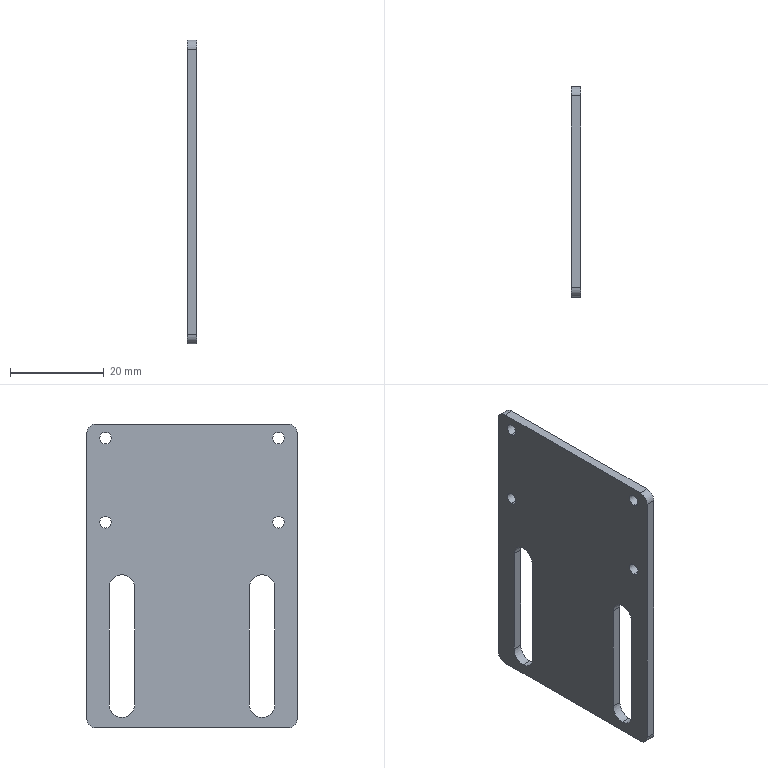Part | SolidWorks | features Fillet 1, FlatPattern 1, HoleWzd 1, ICE 1, SMBaseFlange 1, SheetMetal 1 | 1 solid | 28 faces | box 2 x 45 x 65 mm | volume 5159 mm3 | cylinder 18 | plane 10 | commonest cylinder face diameters 2.5 x8 5.5 x6 4 x4
STEP:
#1=CARTESIAN_POINT('',(-2.,18.5,30.75));
#2=VERTEX_POINT('',#1);
#3=CARTESIAN_POINT('',(-2.,18.5,28.25));
#4=VERTEX_POINT('',#3);
#5=CARTESIAN_POINT('',(-2.,18.5,29.5));
#6=DIRECTION('',(1.,0.,0.));
#7=DIRECTION('',(0.,0.,-1.));
#8=AXIS2_PLACEMENT_3D('',#5,#6,#7);
#9=CIRCLE('',#8,1.25);
#10=EDGE_CURVE('',#2,#4,#9,.T.);
#11=ORIENTED_EDGE('',*,*,#10,.F.);
#12=CARTESIAN_POINT('',(0.,18.5,30.75));
#13=VERTEX_POINT('',#12);
#14=CARTESIAN_POINT('',(0.,18.5,30.75));
#15=DIRECTION('',(1.,0.,0.));
#16=VECTOR('',#15,1000.);
#17=LINE('',#14,#16);
#18=EDGE_CURVE('',#2,#13,#17,.T.);
#19=ORIENTED_EDGE('',*,*,#18,.T.);
#20=CARTESIAN_POINT('',(0.,18.5,28.25));
#21=VERTEX_POINT('',#20);
#22=CARTESIAN_POINT('',(0.,18.5,29.5));
#23=DIRECTION('',(1.,0.,0.));
#24=DIRECTION('',(0.,0.,-1.));
#25=AXIS2_PLACEMENT_3D('',#22,#23,#24);
#26=CIRCLE('',#25,1.25);
#27=EDGE_CURVE('',#13,#21,#26,.T.);
#28=ORIENTED_EDGE('',*,*,#27,.T.);
#29=CARTESIAN_POINT('',(0.,18.5,28.25));
#30=DIRECTION('',(1.,0.,0.));
#31=VECTOR('',#30,1000.);
#32=LINE('',#29,#31);
#33=EDGE_CURVE('',#4,#21,#32,.T.);
#34=ORIENTED_EDGE('',*,*,#33,.F.);
#35=EDGE_LOOP('',(#11,#19,#28,#34));
#36=FACE_OUTER_BOUND('',#35,.T.);
#37=CARTESIAN_POINT('',(0.,18.5,29.5));
#38=DIRECTION('',(1.,0.,0.));
#39=DIRECTION('',(0.,0.,-1.));
#40=AXIS2_PLACEMENT_3D('',#37,#38,#39);
#41=CYLINDRICAL_SURFACE('',#40,1.25);
#42=ADVANCED_FACE('',(#36),#41,.F.);
#43=CARTESIAN_POINT('',(-2.,-18.5,12.75));
#44=VERTEX_POINT('',#43);
#45=CARTESIAN_POINT('',(-2.,-18.5,10.25));
#46=VERTEX_POINT('',#45);
#47=CARTESIAN_POINT('',(-2.,-18.5,11.5));
#48=DIRECTION('',(1.,0.,0.));
#49=DIRECTION('',(0.,0.,-1.));
#50=AXIS2_PLACEMENT_3D('',#47,#48,#49);
#51=CIRCLE('',#50,1.25);
#52=EDGE_CURVE('',#44,#46,#51,.T.);
#53=ORIENTED_EDGE('',*,*,#52,.F.);
#54=CARTESIAN_POINT('',(0.,-18.5,12.75));
#55=VERTEX_POINT('',#54);
#56=CARTESIAN_POINT('',(0.,-18.5,12.75));
#57=DIRECTION('',(1.,0.,0.));
#58=VECTOR('',#57,1000.);
#59=LINE('',#56,#58);
#60=EDGE_CURVE('',#44,#55,#59,.T.);
#61=ORIENTED_EDGE('',*,*,#60,.T.);
#62=CARTESIAN_POINT('',(0.,-18.5,10.25));
#63=VERTEX_POINT('',#62);
#64=CARTESIAN_POINT('',(0.,-18.5,11.5));
#65=DIRECTION('',(1.,0.,0.));
#66=DIRECTION('',(0.,0.,-1.));
#67=AXIS2_PLACEMENT_3D('',#64,#65,#66);
#68=CIRCLE('',#67,1.25);
#69=EDGE_CURVE('',#55,#63,#68,.T.);
#70=ORIENTED_EDGE('',*,*,#69,.T.);
#71=CARTESIAN_POINT('',(0.,-18.5,10.25));
#72=DIRECTION('',(1.,0.,0.));
#73=VECTOR('',#72,1000.);
#74=LINE('',#71,#73);
#75=EDGE_CURVE('',#46,#63,#74,.T.);
#76=ORIENTED_EDGE('',*,*,#75,.F.);
#77=EDGE_LOOP('',(#53,#61,#70,#76));
#78=FACE_OUTER_BOUND('',#77,.T.);
#79=CARTESIAN_POINT('',(0.,-18.5,11.5));
#80=DIRECTION('',(1.,0.,0.));
#81=DIRECTION('',(0.,0.,-1.));
#82=AXIS2_PLACEMENT_3D('',#79,#80,#81);
#83=CYLINDRICAL_SURFACE('',#82,1.25);
#84=ADVANCED_FACE('',(#78),#83,.F.);
#85=CARTESIAN_POINT('',(-2.,18.5,12.75));
#86=VERTEX_POINT('',#85);
#87=CARTESIAN_POINT('',(-2.,18.5,10.25));
#88=VERTEX_POINT('',#87);
#89=CARTESIAN_POINT('',(-2.,18.5,11.5));
#90=DIRECTION('',(1.,0.,0.));
#91=DIRECTION('',(0.,0.,-1.));
#92=AXIS2_PLACEMENT_3D('',#89,#90,#91);
#93=CIRCLE('',#92,1.25);
#94=EDGE_CURVE('',#86,#88,#93,.T.);
#95=ORIENTED_EDGE('',*,*,#94,.F.);
#96=CARTESIAN_POINT('',(0.,18.5,12.75));
#97=VERTEX_POINT('',#96);
#98=CARTESIAN_POINT('',(0.,18.5,12.75));
#99=DIRECTION('',(1.,0.,0.));
#100=VECTOR('',#99,1000.);
#101=LINE('',#98,#100);
#102=EDGE_CURVE('',#86,#97,#101,.T.);
#103=ORIENTED_EDGE('',*,*,#102,.T.);
#104=CARTESIAN_POINT('',(0.,18.5,10.25));
#105=VERTEX_POINT('',#104);
#106=CARTESIAN_POINT('',(0.,18.5,11.5));
#107=DIRECTION('',(1.,0.,0.));
#108=DIRECTION('',(0.,0.,-1.));
#109=AXIS2_PLACEMENT_3D('',#106,#107,#108);
#110=CIRCLE('',#109,1.25);
#111=EDGE_CURVE('',#97,#105,#110,.T.);
#112=ORIENTED_EDGE('',*,*,#111,.T.);
#113=CARTESIAN_POINT('',(0.,18.5,10.25));
#114=DIRECTION('',(1.,0.,0.));
#115=VECTOR('',#114,1000.);
#116=LINE('',#113,#115);
#117=EDGE_CURVE('',#88,#105,#116,.T.);
#118=ORIENTED_EDGE('',*,*,#117,.F.);
#119=EDGE_LOOP('',(#95,#103,#112,#118));
#120=FACE_OUTER_BOUND('',#119,.T.);
#121=CARTESIAN_POINT('',(0.,18.5,11.5));
#122=DIRECTION('',(1.,0.,0.));
#123=DIRECTION('',(0.,0.,-1.));
#124=AXIS2_PLACEMENT_3D('',#121,#122,#123);
#125=CYLINDRICAL_SURFACE('',#124,1.25);
#126=ADVANCED_FACE('',(#120),#125,.F.);
#127=CARTESIAN_POINT('',(-2.,-18.5,30.75));
#128=VERTEX_POINT('',#127);
#129=CARTESIAN_POINT('',(-2.,-18.5,28.25));
#130=VERTEX_POINT('',#129);
#131=CARTESIAN_POINT('',(-2.,-18.5,29.5));
#132=DIRECTION('',(1.,0.,0.));
#133=DIRECTION('',(0.,0.,-1.));
#134=AXIS2_PLACEMENT_3D('',#131,#132,#133);
#135=CIRCLE('',#134,1.25);
#136=EDGE_CURVE('',#128,#130,#135,.T.);
#137=ORIENTED_EDGE('',*,*,#136,.F.);
#138=CARTESIAN_POINT('',(0.,-18.5,30.75));
#139=VERTEX_POINT('',#138);
#140=CARTESIAN_POINT('',(0.,-18.5,30.75));
#141=DIRECTION('',(1.,0.,0.));
#142=VECTOR('',#141,1000.);
#143=LINE('',#140,#142);
#144=EDGE_CURVE('',#128,#139,#143,.T.);
#145=ORIENTED_EDGE('',*,*,#144,.T.);
#146=CARTESIAN_POINT('',(0.,-18.5,28.25));
#147=VERTEX_POINT('',#146);
#148=CARTESIAN_POINT('',(0.,-18.5,29.5));
#149=DIRECTION('',(1.,0.,0.));
#150=DIRECTION('',(0.,0.,-1.));
#151=AXIS2_PLACEMENT_3D('',#148,#149,#150);
#152=CIRCLE('',#151,1.25);
#153=EDGE_CURVE('',#139,#147,#152,.T.);
#154=ORIENTED_EDGE('',*,*,#153,.T.);
#155=CARTESIAN_POINT('',(0.,-18.5,28.25));
#156=DIRECTION('',(1.,0.,0.));
#157=VECTOR('',#156,1000.);
#158=LINE('',#155,#157);
#159=EDGE_CURVE('',#130,#147,#158,.T.);
#160=ORIENTED_EDGE('',*,*,#159,.F.);
#161=EDGE_LOOP('',(#137,#145,#154,#160));
#162=FACE_OUTER_BOUND('',#161,.T.);
#163=CARTESIAN_POINT('',(0.,-18.5,29.5));
#164=DIRECTION('',(1.,0.,0.));
#165=DIRECTION('',(0.,0.,-1.));
#166=AXIS2_PLACEMENT_3D('',#163,#164,#165);
#167=CYLINDRICAL_SURFACE('',#166,1.25);
#168=ADVANCED_FACE('',(#162),#167,.F.);
#169=CARTESIAN_POINT('',(-2.,-12.25,-27.5));
#170=VERTEX_POINT('',#169);
#171=CARTESIAN_POINT('',(-2.,-15.,-30.25));
#172=VERTEX_POINT('',#171);
#173=CARTESIAN_POINT('',(-2.,-15.,-27.5));
#174=DIRECTION('',(-1.,0.,0.));
#175=DIRECTION('',(0.,0.,-1.));
#176=AXIS2_PLACEMENT_3D('',#173,#174,#175);
#177=CIRCLE('',#176,2.75);
#178=EDGE_CURVE('',#170,#172,#177,.T.);
#179=ORIENTED_EDGE('',*,*,#178,.T.);
#180=CARTESIAN_POINT('',(0.,-15.,-30.25));
#181=VERTEX_POINT('',#180);
#182=CARTESIAN_POINT('',(-32.992,-15.,-30.25));
#183=DIRECTION('',(1.,0.,0.));
#184=VECTOR('',#183,1000.);
#185=LINE('',#182,#184);
#186=EDGE_CURVE('',#172,#181,#185,.T.);
#187=ORIENTED_EDGE('',*,*,#186,.T.);
#188=CARTESIAN_POINT('',(0.,-12.25,-27.5));
#189=VERTEX_POINT('',#188);
#190=CARTESIAN_POINT('',(0.,-15.,-27.5));
#191=DIRECTION('',(1.,0.,0.));
#192=DIRECTION('',(0.,0.,1.));
#193=AXIS2_PLACEMENT_3D('',#190,#191,#192);
#194=CIRCLE('',#193,2.75);
#195=EDGE_CURVE('',#181,#189,#194,.T.);
#196=ORIENTED_EDGE('',*,*,#195,.T.);
#197=CARTESIAN_POINT('',(-32.992,-12.25,-27.5));
#198=DIRECTION('',(1.,0.,0.));
#199=VECTOR('',#198,1000.);
#200=LINE('',#197,#199);
#201=EDGE_CURVE('',#170,#189,#200,.T.);
#202=ORIENTED_EDGE('',*,*,#201,.F.);
#203=EDGE_LOOP('',(#179,#187,#196,#202));
#204=FACE_OUTER_BOUND('',#203,.T.);
#205=CARTESIAN_POINT('',(-32.992,-15.,-27.5));
#206=DIRECTION('',(1.,0.,0.));
#207=DIRECTION('',(0.,0.,-1.));
#208=AXIS2_PLACEMENT_3D('',#205,#206,#207);
#209=CYLINDRICAL_SURFACE('',#208,2.75);
#210=ADVANCED_FACE('',(#204),#209,.F.);
#211=CARTESIAN_POINT('',(-2.,17.75,-27.5));
#212=VERTEX_POINT('',#211);
#213=CARTESIAN_POINT('',(-2.,15.,-30.25));
#214=VERTEX_POINT('',#213);
#215=CARTESIAN_POINT('',(-2.,15.,-27.5));
#216=DIRECTION('',(-1.,0.,0.));
#217=DIRECTION('',(0.,0.,-1.));
#218=AXIS2_PLACEMENT_3D('',#215,#216,#217);
#219=CIRCLE('',#218,2.75);
#220=EDGE_CURVE('',#212,#214,#219,.T.);
#221=ORIENTED_EDGE('',*,*,#220,.T.);
#222=CARTESIAN_POINT('',(0.,15.,-30.25));
#223=VERTEX_POINT('',#222);
#224=CARTESIAN_POINT('',(-32.992,15.,-30.25));
#225=DIRECTION('',(1.,0.,0.));
#226=VECTOR('',#225,1000.);
#227=LINE('',#224,#226);
#228=EDGE_CURVE('',#214,#223,#227,.T.);
#229=ORIENTED_EDGE('',*,*,#228,.T.);
#230=CARTESIAN_POINT('',(0.,17.75,-27.5));
#231=VERTEX_POINT('',#230);
#232=CARTESIAN_POINT('',(0.,15.,-27.5));
#233=DIRECTION('',(1.,0.,0.));
#234=DIRECTION('',(0.,0.,-1.));
#235=AXIS2_PLACEMENT_3D('',#232,#233,#234);
#236=CIRCLE('',#235,2.75);
#237=EDGE_CURVE('',#223,#231,#236,.T.);
#238=ORIENTED_EDGE('',*,*,#237,.T.);
#239=CARTESIAN_POINT('',(-32.992,17.75,-27.5));
#240=DIRECTION('',(1.,0.,0.));
#241=VECTOR('',#240,1000.);
#242=LINE('',#239,#241);
#243=EDGE_CURVE('',#212,#231,#242,.T.);
#244=ORIENTED_EDGE('',*,*,#243,.F.);
#245=EDGE_LOOP('',(#221,#229,#238,#244));
#246=FACE_OUTER_BOUND('',#245,.T.);
#247=CARTESIAN_POINT('',(-32.992,15.,-27.5));
#248=DIRECTION('',(1.,0.,0.));
#249=DIRECTION('',(0.,0.,-1.));
#250=AXIS2_PLACEMENT_3D('',#247,#248,#249);
#251=CYLINDRICAL_SURFACE('',#250,2.75);
#252=ADVANCED_FACE('',(#246),#251,.F.);
#253=CARTESIAN_POINT('',(-2.,18.5,29.5));
#254=DIRECTION('',(1.,0.,0.));
#255=DIRECTION('',(0.,0.,-1.));
#256=AXIS2_PLACEMENT_3D('',#253,#254,#255);
#257=CIRCLE('',#256,1.25);
#258=EDGE_CURVE('',#4,#2,#257,.T.);
#259=ORIENTED_EDGE('',*,*,#258,.T.);
#260=ORIENTED_EDGE('',*,*,#10,.T.);
#261=EDGE_LOOP('',(#259,#260));
#262=FACE_BOUND('',#261,.T.);
#263=CARTESIAN_POINT('',(-2.,-18.5,11.5));
#264=DIRECTION('',(1.,0.,0.));
#265=DIRECTION('',(0.,0.,-1.));
#266=AXIS2_PLACEMENT_3D('',#263,#264,#265);
#267=CIRCLE('',#266,1.25);
#268=EDGE_CURVE('',#46,#44,#267,.T.);
#269=ORIENTED_EDGE('',*,*,#268,.T.);
#270=ORIENTED_EDGE('',*,*,#52,.T.);
#271=EDGE_LOOP('',(#269,#270));
#272=FACE_BOUND('',#271,.T.);
#273=CARTESIAN_POINT('',(-2.,18.5,11.5));
#274=DIRECTION('',(1.,0.,0.));
#275=DIRECTION('',(0.,0.,-1.));
#276=AXIS2_PLACEMENT_3D('',#273,#274,#275);
#277=CIRCLE('',#276,1.25);
#278=EDGE_CURVE('',#88,#86,#277,.T.);
#279=ORIENTED_EDGE('',*,*,#278,.T.);
#280=ORIENTED_EDGE('',*,*,#94,.T.);
#281=EDGE_LOOP('',(#279,#280));
#282=FACE_BOUND('',#281,.T.);
#283=CARTESIAN_POINT('',(-2.,-18.5,29.5));
#284=DIRECTION('',(1.,0.,0.));
#285=DIRECTION('',(0.,0.,-1.));
#286=AXIS2_PLACEMENT_3D('',#283,#284,#285);
#287=CIRCLE('',#286,1.25);
#288=EDGE_CURVE('',#130,#128,#287,.T.);
#289=ORIENTED_EDGE('',*,*,#288,.T.);
#290=ORIENTED_EDGE('',*,*,#136,.T.);
#291=EDGE_LOOP('',(#289,#290));
#292=FACE_BOUND('',#291,.T.);
#293=CARTESIAN_POINT('',(-2.,-12.25,-2.5));
#294=VERTEX_POINT('',#293);
#295=CARTESIAN_POINT('',(-2.,-12.25,-2.5));
#296=DIRECTION('',(0.,0.,-1.));
#297=VECTOR('',#296,1000.);
#298=LINE('',#295,#297);
#299=EDGE_CURVE('',#294,#170,#298,.T.);
#300=ORIENTED_EDGE('',*,*,#299,.F.);
#301=CARTESIAN_POINT('',(-2.,-17.75,-2.5));
#302=VERTEX_POINT('',#301);
#303=CARTESIAN_POINT('',(-2.,-15.,-2.5));
#304=DIRECTION('',(-1.,0.,0.));
#305=DIRECTION('',(0.,0.,-1.));
#306=AXIS2_PLACEMENT_3D('',#303,#304,#305);
#307=CIRCLE('',#306,2.75);
#308=EDGE_CURVE('',#302,#294,#307,.T.);
#309=ORIENTED_EDGE('',*,*,#308,.F.);
#310=CARTESIAN_POINT('',(-2.,-17.75,-27.5));
#311=VERTEX_POINT('',#310);
#312=CARTESIAN_POINT('',(-2.,-17.75,-2.5));
#313=DIRECTION('',(0.,0.,1.));
#314=VECTOR('',#313,1000.);
#315=LINE('',#312,#314);
#316=EDGE_CURVE('',#311,#302,#315,.T.);
#317=ORIENTED_EDGE('',*,*,#316,.F.);
#318=CARTESIAN_POINT('',(-2.,-15.,-27.5));
#319=DIRECTION('',(-1.,0.,0.));
#320=DIRECTION('',(0.,0.,-1.));
#321=AXIS2_PLACEMENT_3D('',#318,#319,#320);
#322=CIRCLE('',#321,2.75);
#323=EDGE_CURVE('',#172,#311,#322,.T.);
#324=ORIENTED_EDGE('',*,*,#323,.F.);
#325=ORIENTED_EDGE('',*,*,#178,.F.);
#326=EDGE_LOOP('',(#300,#309,#317,#324,#325));
#327=FACE_BOUND('',#326,.T.);
#328=CARTESIAN_POINT('',(-2.,17.75,-2.5));
#329=VERTEX_POINT('',#328);
#330=CARTESIAN_POINT('',(-2.,17.75,-2.5));
#331=DIRECTION('',(0.,0.,-1.));
#332=VECTOR('',#331,1000.);
#333=LINE('',#330,#332);
#334=EDGE_CURVE('',#329,#212,#333,.T.);
#335=ORIENTED_EDGE('',*,*,#334,.F.);
#336=CARTESIAN_POINT('',(-2.,12.25,-2.5));
#337=VERTEX_POINT('',#336);
#338=CARTESIAN_POINT('',(-2.,15.,-2.5));
#339=DIRECTION('',(-1.,0.,0.));
#340=DIRECTION('',(0.,0.,-1.));
#341=AXIS2_PLACEMENT_3D('',#338,#339,#340);
#342=CIRCLE('',#341,2.75);
#343=EDGE_CURVE('',#337,#329,#342,.T.);
#344=ORIENTED_EDGE('',*,*,#343,.F.);
#345=CARTESIAN_POINT('',(-2.,12.25,-27.5));
#346=VERTEX_POINT('',#345);
#347=CARTESIAN_POINT('',(-2.,12.25,-2.5));
#348=DIRECTION('',(0.,0.,1.));
#349=VECTOR('',#348,1000.);
#350=LINE('',#347,#349);
#351=EDGE_CURVE('',#346,#337,#350,.T.);
#352=ORIENTED_EDGE('',*,*,#351,.F.);
#353=CARTESIAN_POINT('',(-2.,15.,-27.5));
#354=DIRECTION('',(-1.,0.,0.));
#355=DIRECTION('',(0.,0.,-1.));
#356=AXIS2_PLACEMENT_3D('',#353,#354,#355);
#357=CIRCLE('',#356,2.75);
#358=EDGE_CURVE('',#214,#346,#357,.T.);
#359=ORIENTED_EDGE('',*,*,#358,.F.);
#360=ORIENTED_EDGE('',*,*,#220,.F.);
#361=EDGE_LOOP('',(#335,#344,#352,#359,#360));
#362=FACE_BOUND('',#361,.T.);
#363=CARTESIAN_POINT('',(-2.,20.5,32.5));
#364=VERTEX_POINT('',#363);
#365=CARTESIAN_POINT('',(-2.,-20.5,32.5));
#366=VERTEX_POINT('',#365);
#367=CARTESIAN_POINT('',(-2.,22.5,32.5));
#368=DIRECTION('',(0.,-1.,0.));
#369=VECTOR('',#368,1000.);
#370=LINE('',#367,#369);
#371=EDGE_CURVE('',#364,#366,#370,.T.);
#372=ORIENTED_EDGE('',*,*,#371,.F.);
#373=CARTESIAN_POINT('',(-2.,22.5,30.5));
#374=VERTEX_POINT('',#373);
#375=CARTESIAN_POINT('',(-2.,20.5,30.5));
#376=DIRECTION('',(-1.,0.,0.));
#377=DIRECTION('',(0.,0.,-1.));
#378=AXIS2_PLACEMENT_3D('',#375,#376,#377);
#379=CIRCLE('',#378,2.);
#380=EDGE_CURVE('',#364,#374,#379,.T.);
#381=ORIENTED_EDGE('',*,*,#380,.T.);
#382=CARTESIAN_POINT('',(-2.,22.5,-30.5));
#383=VERTEX_POINT('',#382);
#384=CARTESIAN_POINT('',(-2.,22.5,-32.5));
#385=DIRECTION('',(0.,0.,1.));
#386=VECTOR('',#385,1000.);
#387=LINE('',#384,#386);
#388=EDGE_CURVE('',#383,#374,#387,.T.);
#389=ORIENTED_EDGE('',*,*,#388,.F.);
#390=CARTESIAN_POINT('',(-2.,20.5,-32.5));
#391=VERTEX_POINT('',#390);
#392=CARTESIAN_POINT('',(-2.,20.5,-30.5));
#393=DIRECTION('',(-1.,0.,0.));
#394=DIRECTION('',(0.,0.,-1.));
#395=AXIS2_PLACEMENT_3D('',#392,#393,#394);
#396=CIRCLE('',#395,2.);
#397=EDGE_CURVE('',#383,#391,#396,.T.);
#398=ORIENTED_EDGE('',*,*,#397,.T.);
#399=CARTESIAN_POINT('',(-2.,-20.5,-32.5));
#400=VERTEX_POINT('',#399);
#401=CARTESIAN_POINT('',(-2.,22.5,-32.5));
#402=DIRECTION('',(0.,-1.,0.));
#403=VECTOR('',#402,1000.);
#404=LINE('',#401,#403);
#405=EDGE_CURVE('',#391,#400,#404,.T.);
#406=ORIENTED_EDGE('',*,*,#405,.T.);
#407=CARTESIAN_POINT('',(-2.,-22.5,-30.5));
#408=VERTEX_POINT('',#407);
#409=CARTESIAN_POINT('',(-2.,-20.5,-30.5));
#410=DIRECTION('',(-1.,0.,0.));
#411=DIRECTION('',(0.,0.,-1.));
#412=AXIS2_PLACEMENT_3D('',#409,#410,#411);
#413=CIRCLE('',#412,2.);
#414=EDGE_CURVE('',#400,#408,#413,.T.);
#415=ORIENTED_EDGE('',*,*,#414,.T.);
#416=CARTESIAN_POINT('',(-2.,-22.5,30.5));
#417=VERTEX_POINT('',#416);
#418=CARTESIAN_POINT('',(-2.,-22.5,-32.5));
#419=DIRECTION('',(0.,0.,1.));
#420=VECTOR('',#419,1000.);
#421=LINE('',#418,#420);
#422=EDGE_CURVE('',#408,#417,#421,.T.);
#423=ORIENTED_EDGE('',*,*,#422,.T.);
#424=CARTESIAN_POINT('',(-2.,-20.5,30.5));
#425=DIRECTION('',(-1.,0.,0.));
#426=DIRECTION('',(0.,0.,-1.));
#427=AXIS2_PLACEMENT_3D('',#424,#425,#426);
#428=CIRCLE('',#427,2.);
#429=EDGE_CURVE('',#417,#366,#428,.T.);
#430=ORIENTED_EDGE('',*,*,#429,.T.);
#431=EDGE_LOOP('',(#372,#381,#389,#398,#406,#415,#423,#430));
#432=FACE_OUTER_BOUND('',#431,.T.);
#433=CARTESIAN_POINT('',(-2.,22.5,-32.5));
#434=DIRECTION('',(1.,0.,0.));
#435=DIRECTION('',(0.,0.,-1.));
#436=AXIS2_PLACEMENT_3D('',#433,#434,#435);
#437=PLANE('',#436);
#438=ADVANCED_FACE('',(#262,#272,#282,#292,#327,#362,#432),#437,.F.);
#439=CARTESIAN_POINT('',(0.,20.5,32.5));
#440=VERTEX_POINT('',#439);
#441=CARTESIAN_POINT('',(0.,-20.5,32.5));
#442=VERTEX_POINT('',#441);
#443=CARTESIAN_POINT('',(0.,22.5,32.5));
#444=DIRECTION('',(0.,-1.,0.));
#445=VECTOR('',#444,1000.);
#446=LINE('',#443,#445);
#447=EDGE_CURVE('',#440,#442,#446,.T.);
#448=ORIENTED_EDGE('',*,*,#447,.F.);
#449=CARTESIAN_POINT('',(0.,20.5,32.5));
#450=DIRECTION('',(-1.,0.,0.));
#451=VECTOR('',#450,1000.);
#452=LINE('',#449,#451);
#453=EDGE_CURVE('',#440,#364,#452,.T.);
#454=ORIENTED_EDGE('',*,*,#453,.T.);
#455=ORIENTED_EDGE('',*,*,#371,.T.);
#456=CARTESIAN_POINT('',(0.,-20.5,32.5));
#457=DIRECTION('',(1.,0.,0.));
#458=VECTOR('',#457,1000.);
#459=LINE('',#456,#458);
#460=EDGE_CURVE('',#366,#442,#459,.T.);
#461=ORIENTED_EDGE('',*,*,#460,.T.);
#462=EDGE_LOOP('',(#448,#454,#455,#461));
#463=FACE_OUTER_BOUND('',#462,.T.);
#464=CARTESIAN_POINT('',(0.,22.5,32.5));
#465=DIRECTION('',(0.,0.,1.));
#466=DIRECTION('',(1.,0.,0.));
#467=AXIS2_PLACEMENT_3D('',#464,#465,#466);
#468=PLANE('',#467);
#469=ADVANCED_FACE('',(#463),#468,.T.);
#470=CARTESIAN_POINT('',(0.,18.5,29.5));
#471=DIRECTION('',(1.,0.,0.));
#472=DIRECTION('',(0.,0.,-1.));
#473=AXIS2_PLACEMENT_3D('',#470,#471,#472);
#474=CIRCLE('',#473,1.25);
#475=EDGE_CURVE('',#21,#13,#474,.T.);
#476=ORIENTED_EDGE('',*,*,#475,.F.);
#477=ORIENTED_EDGE('',*,*,#27,.F.);
#478=EDGE_LOOP('',(#476,#477));
#479=FACE_BOUND('',#478,.T.);
#480=CARTESIAN_POINT('',(0.,-18.5,11.5));
#481=DIRECTION('',(1.,0.,0.));
#482=DIRECTION('',(0.,0.,-1.));
#483=AXIS2_PLACEMENT_3D('',#480,#481,#482);
#484=CIRCLE('',#483,1.25);
#485=EDGE_CURVE('',#63,#55,#484,.T.);
#486=ORIENTED_EDGE('',*,*,#485,.F.);
#487=ORIENTED_EDGE('',*,*,#69,.F.);
#488=EDGE_LOOP('',(#486,#487));
#489=FACE_BOUND('',#488,.T.);
#490=CARTESIAN_POINT('',(0.,18.5,11.5));
#491=DIRECTION('',(1.,0.,0.));
#492=DIRECTION('',(0.,0.,-1.));
#493=AXIS2_PLACEMENT_3D('',#490,#491,#492);
#494=CIRCLE('',#493,1.25);
#495=EDGE_CURVE('',#105,#97,#494,.T.);
#496=ORIENTED_EDGE('',*,*,#495,.F.);
#497=ORIENTED_EDGE('',*,*,#111,.F.);
#498=EDGE_LOOP('',(#496,#497));
#499=FACE_BOUND('',#498,.T.);
#500=CARTESIAN_POINT('',(0.,-18.5,29.5));
#501=DIRECTION('',(1.,0.,0.));
#502=DIRECTION('',(0.,0.,-1.));
#503=AXIS2_PLACEMENT_3D('',#500,#501,#502);
#504=CIRCLE('',#503,1.25);
#505=EDGE_CURVE('',#147,#139,#504,.T.);
#506=ORIENTED_EDGE('',*,*,#505,.F.);
#507=ORIENTED_EDGE('',*,*,#153,.F.);
#508=EDGE_LOOP('',(#506,#507));
#509=FACE_BOUND('',#508,.T.);
#510=CARTESIAN_POINT('',(0.,-12.25,-2.5));
#511=VERTEX_POINT('',#510);
#512=CARTESIAN_POINT('',(0.,-17.75,-2.5));
#513=VERTEX_POINT('',#512);
#514=CARTESIAN_POINT('',(0.,-15.,-2.5));
#515=DIRECTION('',(1.,0.,0.));
#516=DIRECTION('',(0.,0.,1.));
#517=AXIS2_PLACEMENT_3D('',#514,#515,#516);
#518=CIRCLE('',#517,2.75);
#519=EDGE_CURVE('',#511,#513,#518,.T.);
#520=ORIENTED_EDGE('',*,*,#519,.F.);
#521=CARTESIAN_POINT('',(0.,-12.25,-2.5));
#522=DIRECTION('',(0.,0.,1.));
#523=VECTOR('',#522,1000.);
#524=LINE('',#521,#523);
#525=EDGE_CURVE('',#189,#511,#524,.T.);
#526=ORIENTED_EDGE('',*,*,#525,.F.);
#527=ORIENTED_EDGE('',*,*,#195,.F.);
#528=CARTESIAN_POINT('',(0.,-17.75,-27.5));
#529=VERTEX_POINT('',#528);
#530=CARTESIAN_POINT('',(0.,-15.,-27.5));
#531=DIRECTION('',(1.,0.,0.));
#532=DIRECTION('',(0.,0.,1.));
#533=AXIS2_PLACEMENT_3D('',#530,#531,#532);
#534=CIRCLE('',#533,2.75);
#535=EDGE_CURVE('',#529,#181,#534,.T.);
#536=ORIENTED_EDGE('',*,*,#535,.F.);
#537=CARTESIAN_POINT('',(0.,-17.75,-2.5));
#538=DIRECTION('',(0.,0.,-1.));
#539=VECTOR('',#538,1000.);
#540=LINE('',#537,#539);
#541=EDGE_CURVE('',#513,#529,#540,.T.);
#542=ORIENTED_EDGE('',*,*,#541,.F.);
#543=EDGE_LOOP('',(#520,#526,#527,#536,#542));
#544=FACE_BOUND('',#543,.T.);
#545=CARTESIAN_POINT('',(0.,17.75,-2.5));
#546=VERTEX_POINT('',#545);
#547=CARTESIAN_POINT('',(0.,12.25,-2.5));
#548=VERTEX_POINT('',#547);
#549=CARTESIAN_POINT('',(0.,15.,-2.5));
#550=DIRECTION('',(1.,0.,0.));
#551=DIRECTION('',(0.,0.,-1.));
#552=AXIS2_PLACEMENT_3D('',#549,#550,#551);
#553=CIRCLE('',#552,2.75);
#554=EDGE_CURVE('',#546,#548,#553,.T.);
#555=ORIENTED_EDGE('',*,*,#554,.F.);
#556=CARTESIAN_POINT('',(0.,17.75,-2.5));
#557=DIRECTION('',(0.,0.,1.));
#558=VECTOR('',#557,1000.);
#559=LINE('',#556,#558);
#560=EDGE_CURVE('',#231,#546,#559,.T.);
#561=ORIENTED_EDGE('',*,*,#560,.F.);
#562=ORIENTED_EDGE('',*,*,#237,.F.);
#563=CARTESIAN_POINT('',(0.,12.25,-27.5));
#564=VERTEX_POINT('',#563);
#565=CARTESIAN_POINT('',(0.,15.,-27.5));
#566=DIRECTION('',(1.,0.,0.));
#567=DIRECTION('',(0.,0.,-1.));
#568=AXIS2_PLACEMENT_3D('',#565,#566,#567);
#569=CIRCLE('',#568,2.75);
#570=EDGE_CURVE('',#564,#223,#569,.T.);
#571=ORIENTED_EDGE('',*,*,#570,.F.);
#572=CARTESIAN_POINT('',(0.,12.25,-2.5));
#573=DIRECTION('',(0.,0.,-1.));
#574=VECTOR('',#573,1000.);
#575=LINE('',#572,#574);
#576=EDGE_CURVE('',#548,#564,#575,.T.);
#577=ORIENTED_EDGE('',*,*,#576,.F.);
#578=EDGE_LOOP('',(#555,#561,#562,#571,#577));
#579=FACE_BOUND('',#578,.T.);
#580=CARTESIAN_POINT('',(0.,22.5,-30.5));
#581=VERTEX_POINT('',#580);
#582=CARTESIAN_POINT('',(0.,22.5,30.5));
#583=VERTEX_POINT('',#582);
#584=CARTESIAN_POINT('',(0.,22.5,-32.5));
#585=DIRECTION('',(0.,0.,1.));
#586=VECTOR('',#585,1000.);
#587=LINE('',#584,#586);
#588=EDGE_CURVE('',#581,#583,#587,.T.);
#589=ORIENTED_EDGE('',*,*,#588,.T.);
#590=CARTESIAN_POINT('',(0.,20.5,30.5));
#591=DIRECTION('',(1.,0.,0.));
#592=DIRECTION('',(0.,0.,-1.));
#593=AXIS2_PLACEMENT_3D('',#590,#591,#592);
#594=CIRCLE('',#593,2.);
#595=EDGE_CURVE('',#583,#440,#594,.T.);
#596=ORIENTED_EDGE('',*,*,#595,.T.);
#597=ORIENTED_EDGE('',*,*,#447,.T.);
#598=CARTESIAN_POINT('',(0.,-22.5,30.5));
#599=VERTEX_POINT('',#598);
#600=CARTESIAN_POINT('',(0.,-20.5,30.5));
#601=DIRECTION('',(1.,0.,0.));
#602=DIRECTION('',(0.,0.,-1.));
#603=AXIS2_PLACEMENT_3D('',#600,#601,#602);
#604=CIRCLE('',#603,2.);
#605=EDGE_CURVE('',#442,#599,#604,.T.);
#606=ORIENTED_EDGE('',*,*,#605,.T.);
#607=CARTESIAN_POINT('',(0.,-22.5,-30.5));
#608=VERTEX_POINT('',#607);
#609=CARTESIAN_POINT('',(0.,-22.5,-32.5));
#610=DIRECTION('',(0.,0.,1.));
#611=VECTOR('',#610,1000.);
#612=LINE('',#609,#611);
#613=EDGE_CURVE('',#608,#599,#612,.T.);
#614=ORIENTED_EDGE('',*,*,#613,.F.);
#615=CARTESIAN_POINT('',(0.,-20.5,-32.5));
#616=VERTEX_POINT('',#615);
#617=CARTESIAN_POINT('',(0.,-20.5,-30.5));
#618=DIRECTION('',(1.,0.,0.));
#619=DIRECTION('',(0.,0.,-1.));
#620=AXIS2_PLACEMENT_3D('',#617,#618,#619);
#621=CIRCLE('',#620,2.);
#622=EDGE_CURVE('',#608,#616,#621,.T.);
#623=ORIENTED_EDGE('',*,*,#622,.T.);
#624=CARTESIAN_POINT('',(0.,20.5,-32.5));
#625=VERTEX_POINT('',#624);
#626=CARTESIAN_POINT('',(0.,22.5,-32.5));
#627=DIRECTION('',(0.,-1.,0.));
#628=VECTOR('',#627,1000.);
#629=LINE('',#626,#628);
#630=EDGE_CURVE('',#625,#616,#629,.T.);
#631=ORIENTED_EDGE('',*,*,#630,.F.);
#632=CARTESIAN_POINT('',(0.,20.5,-30.5));
#633=DIRECTION('',(1.,0.,0.));
#634=DIRECTION('',(0.,0.,-1.));
#635=AXIS2_PLACEMENT_3D('',#632,#633,#634);
#636=CIRCLE('',#635,2.);
#637=EDGE_CURVE('',#625,#581,#636,.T.);
#638=ORIENTED_EDGE('',*,*,#637,.T.);
#639=EDGE_LOOP('',(#589,#596,#597,#606,#614,#623,#631,#638));
#640=FACE_OUTER_BOUND('',#639,.T.);
#641=CARTESIAN_POINT('',(0.,22.5,-32.5));
#642=DIRECTION('',(1.,0.,0.));
#643=DIRECTION('',(0.,0.,-1.));
#644=AXIS2_PLACEMENT_3D('',#641,#642,#643);
#645=PLANE('',#644);
#646=ADVANCED_FACE('',(#479,#489,#499,#509,#544,#579,#640),#645,.T.);
#647=ORIENTED_EDGE('',*,*,#405,.F.);
#648=CARTESIAN_POINT('',(-2.,20.5,-32.5));
#649=DIRECTION('',(1.,0.,0.));
#650=VECTOR('',#649,1000.);
#651=LINE('',#648,#650);
#652=EDGE_CURVE('',#391,#625,#651,.T.);
#653=ORIENTED_EDGE('',*,*,#652,.T.);
#654=ORIENTED_EDGE('',*,*,#630,.T.);
#655=CARTESIAN_POINT('',(-2.,-20.5,-32.5));
#656=DIRECTION('',(-1.,0.,0.));
#657=VECTOR('',#656,1000.);
#658=LINE('',#655,#657);
#659=EDGE_CURVE('',#616,#400,#658,.T.);
#660=ORIENTED_EDGE('',*,*,#659,.T.);
#661=EDGE_LOOP('',(#647,#653,#654,#660));
#662=FACE_OUTER_BOUND('',#661,.T.);
#663=CARTESIAN_POINT('',(-2.,22.5,-32.5));
#664=DIRECTION('',(0.,0.,-1.));
#665=DIRECTION('',(-1.,0.,0.));
#666=AXIS2_PLACEMENT_3D('',#663,#664,#665);
#667=PLANE('',#666);
#668=ADVANCED_FACE('',(#662),#667,.T.);
#669=ORIENTED_EDGE('',*,*,#388,.T.);
#670=CARTESIAN_POINT('',(0.,22.5,30.5));
#671=DIRECTION('',(1.,0.,0.));
#672=VECTOR('',#671,1000.);
#673=LINE('',#670,#672);
#674=EDGE_CURVE('',#374,#583,#673,.T.);
#675=ORIENTED_EDGE('',*,*,#674,.T.);
#676=ORIENTED_EDGE('',*,*,#588,.F.);
#677=CARTESIAN_POINT('',(0.,22.5,-30.5));
#678=DIRECTION('',(-1.,0.,0.));
#679=VECTOR('',#678,1000.);
#680=LINE('',#677,#679);
#681=EDGE_CURVE('',#581,#383,#680,.T.);
#682=ORIENTED_EDGE('',*,*,#681,.T.);
#683=EDGE_LOOP('',(#669,#675,#676,#682));
#684=FACE_OUTER_BOUND('',#683,.T.);
#685=CARTESIAN_POINT('',(0.,22.5,0.));
#686=DIRECTION('',(0.,1.,0.));
#687=DIRECTION('',(1.,0.,0.));
#688=AXIS2_PLACEMENT_3D('',#685,#686,#687);
#689=PLANE('',#688);
#690=ADVANCED_FACE('',(#684),#689,.T.);
#691=ORIENTED_EDGE('',*,*,#613,.T.);
#692=CARTESIAN_POINT('',(-2.,-22.5,30.5));
#693=DIRECTION('',(-1.,0.,0.));
#694=VECTOR('',#693,1000.);
#695=LINE('',#692,#694);
#696=EDGE_CURVE('',#599,#417,#695,.T.);
#697=ORIENTED_EDGE('',*,*,#696,.T.);
#698=ORIENTED_EDGE('',*,*,#422,.F.);
#699=CARTESIAN_POINT('',(0.,-22.5,-30.5));
#700=DIRECTION('',(1.,0.,0.));
#701=VECTOR('',#700,1000.);
#702=LINE('',#699,#701);
#703=EDGE_CURVE('',#408,#608,#702,.T.);
#704=ORIENTED_EDGE('',*,*,#703,.T.);
#705=EDGE_LOOP('',(#691,#697,#698,#704));
#706=FACE_OUTER_BOUND('',#705,.T.);
#707=CARTESIAN_POINT('',(0.,-22.5,0.));
#708=DIRECTION('',(0.,1.,0.));
#709=DIRECTION('',(1.,0.,0.));
#710=AXIS2_PLACEMENT_3D('',#707,#708,#709);
#711=PLANE('',#710);
#712=ADVANCED_FACE('',(#706),#711,.F.);
#713=ORIENTED_EDGE('',*,*,#343,.T.);
#714=CARTESIAN_POINT('',(-32.992,17.75,-2.5));
#715=DIRECTION('',(1.,0.,0.));
#716=VECTOR('',#715,1000.);
#717=LINE('',#714,#716);
#718=EDGE_CURVE('',#329,#546,#717,.T.);
#719=ORIENTED_EDGE('',*,*,#718,.T.);
#720=ORIENTED_EDGE('',*,*,#554,.T.);
#721=CARTESIAN_POINT('',(-32.992,12.25,-2.5));
#722=DIRECTION('',(1.,0.,0.));
#723=VECTOR('',#722,1000.);
#724=LINE('',#721,#723);
#725=EDGE_CURVE('',#337,#548,#724,.T.);
#726=ORIENTED_EDGE('',*,*,#725,.F.);
#727=EDGE_LOOP('',(#713,#719,#720,#726));
#728=FACE_OUTER_BOUND('',#727,.T.);
#729=CARTESIAN_POINT('',(-32.992,15.,-2.5));
#730=DIRECTION('',(1.,0.,0.));
#731=DIRECTION('',(0.,0.,-1.));
#732=AXIS2_PLACEMENT_3D('',#729,#730,#731);
#733=CYLINDRICAL_SURFACE('',#732,2.75);
#734=ADVANCED_FACE('',(#728),#733,.F.);
#735=ORIENTED_EDGE('',*,*,#334,.T.);
#736=ORIENTED_EDGE('',*,*,#243,.T.);
#737=ORIENTED_EDGE('',*,*,#560,.T.);
#738=ORIENTED_EDGE('',*,*,#718,.F.);
#739=EDGE_LOOP('',(#735,#736,#737,#738));
#740=FACE_OUTER_BOUND('',#739,.T.);
#741=CARTESIAN_POINT('',(-32.992,17.75,-2.5));
#742=DIRECTION('',(0.,1.,0.));
#743=DIRECTION('',(0.,0.,1.));
#744=AXIS2_PLACEMENT_3D('',#741,#742,#743);
#745=PLANE('',#744);
#746=ADVANCED_FACE('',(#740),#745,.F.);
#747=ORIENTED_EDGE('',*,*,#228,.F.);
#748=ORIENTED_EDGE('',*,*,#358,.T.);
#749=CARTESIAN_POINT('',(-32.992,12.25,-27.5));
#750=DIRECTION('',(1.,0.,0.));
#751=VECTOR('',#750,1000.);
#752=LINE('',#749,#751);
#753=EDGE_CURVE('',#346,#564,#752,.T.);
#754=ORIENTED_EDGE('',*,*,#753,.T.);
#755=ORIENTED_EDGE('',*,*,#570,.T.);
#756=EDGE_LOOP('',(#747,#748,#754,#755));
#757=FACE_OUTER_BOUND('',#756,.T.);
#758=CARTESIAN_POINT('',(-32.992,15.,-27.5));
#759=DIRECTION('',(1.,0.,0.));
#760=DIRECTION('',(0.,0.,-1.));
#761=AXIS2_PLACEMENT_3D('',#758,#759,#760);
#762=CYLINDRICAL_SURFACE('',#761,2.75);
#763=ADVANCED_FACE('',(#757),#762,.F.);
#764=ORIENTED_EDGE('',*,*,#351,.T.);
#765=ORIENTED_EDGE('',*,*,#725,.T.);
#766=ORIENTED_EDGE('',*,*,#576,.T.);
#767=ORIENTED_EDGE('',*,*,#753,.F.);
#768=EDGE_LOOP('',(#764,#765,#766,#767));
#769=FACE_OUTER_BOUND('',#768,.T.);
#770=CARTESIAN_POINT('',(-32.992,12.25,-2.5));
#771=DIRECTION('',(0.,-1.,0.));
#772=DIRECTION('',(0.,0.,-1.));
#773=AXIS2_PLACEMENT_3D('',#770,#771,#772);
#774=PLANE('',#773);
#775=ADVANCED_FACE('',(#769),#774,.F.);
#776=ORIENTED_EDGE('',*,*,#308,.T.);
#777=CARTESIAN_POINT('',(-32.992,-12.25,-2.5));
#778=DIRECTION('',(1.,0.,0.));
#779=VECTOR('',#778,1000.);
#780=LINE('',#777,#779);
#781=EDGE_CURVE('',#294,#511,#780,.T.);
#782=ORIENTED_EDGE('',*,*,#781,.T.);
#783=ORIENTED_EDGE('',*,*,#519,.T.);
#784=CARTESIAN_POINT('',(-32.992,-17.75,-2.5));
#785=DIRECTION('',(1.,0.,0.));
#786=VECTOR('',#785,1000.);
#787=LINE('',#784,#786);
#788=EDGE_CURVE('',#302,#513,#787,.T.);
#789=ORIENTED_EDGE('',*,*,#788,.F.);
#790=EDGE_LOOP('',(#776,#782,#783,#789));
#791=FACE_OUTER_BOUND('',#790,.T.);
#792=CARTESIAN_POINT('',(-32.992,-15.,-2.5));
#793=DIRECTION('',(1.,0.,0.));
#794=DIRECTION('',(0.,0.,-1.));
#795=AXIS2_PLACEMENT_3D('',#792,#793,#794);
#796=CYLINDRICAL_SURFACE('',#795,2.75);
#797=ADVANCED_FACE('',(#791),#796,.F.);
#798=ORIENTED_EDGE('',*,*,#299,.T.);
#799=ORIENTED_EDGE('',*,*,#201,.T.);
#800=ORIENTED_EDGE('',*,*,#525,.T.);
#801=ORIENTED_EDGE('',*,*,#781,.F.);
#802=EDGE_LOOP('',(#798,#799,#800,#801));
#803=FACE_OUTER_BOUND('',#802,.T.);
#804=CARTESIAN_POINT('',(-32.992,-12.25,-2.5));
#805=DIRECTION('',(0.,1.,0.));
#806=DIRECTION('',(0.,0.,1.));
#807=AXIS2_PLACEMENT_3D('',#804,#805,#806);
#808=PLANE('',#807);
#809=ADVANCED_FACE('',(#803),#808,.F.);
#810=ORIENTED_EDGE('',*,*,#186,.F.);
#811=ORIENTED_EDGE('',*,*,#323,.T.);
#812=CARTESIAN_POINT('',(-32.992,-17.75,-27.5));
#813=DIRECTION('',(1.,0.,0.));
#814=VECTOR('',#813,1000.);
#815=LINE('',#812,#814);
#816=EDGE_CURVE('',#311,#529,#815,.T.);
#817=ORIENTED_EDGE('',*,*,#816,.T.);
#818=ORIENTED_EDGE('',*,*,#535,.T.);
#819=EDGE_LOOP('',(#810,#811,#817,#818));
#820=FACE_OUTER_BOUND('',#819,.T.);
#821=CARTESIAN_POINT('',(-32.992,-15.,-27.5));
#822=DIRECTION('',(1.,0.,0.));
#823=DIRECTION('',(0.,0.,-1.));
#824=AXIS2_PLACEMENT_3D('',#821,#822,#823);
#825=CYLINDRICAL_SURFACE('',#824,2.75);
#826=ADVANCED_FACE('',(#820),#825,.F.);
#827=ORIENTED_EDGE('',*,*,#316,.T.);
#828=ORIENTED_EDGE('',*,*,#788,.T.);
#829=ORIENTED_EDGE('',*,*,#541,.T.);
#830=ORIENTED_EDGE('',*,*,#816,.F.);
#831=EDGE_LOOP('',(#827,#828,#829,#830));
#832=FACE_OUTER_BOUND('',#831,.T.);
#833=CARTESIAN_POINT('',(-32.992,-17.75,-2.5));
#834=DIRECTION('',(0.,-1.,0.));
#835=DIRECTION('',(0.,0.,-1.));
#836=AXIS2_PLACEMENT_3D('',#833,#834,#835);
#837=PLANE('',#836);
#838=ADVANCED_FACE('',(#832),#837,.F.);
#839=ORIENTED_EDGE('',*,*,#144,.F.);
#840=ORIENTED_EDGE('',*,*,#288,.F.);
#841=ORIENTED_EDGE('',*,*,#159,.T.);
#842=ORIENTED_EDGE('',*,*,#505,.T.);
#843=EDGE_LOOP('',(#839,#840,#841,#842));
#844=FACE_OUTER_BOUND('',#843,.T.);
#845=CARTESIAN_POINT('',(0.,-18.5,29.5));
#846=DIRECTION('',(1.,0.,0.));
#847=DIRECTION('',(0.,0.,-1.));
#848=AXIS2_PLACEMENT_3D('',#845,#846,#847);
#849=CYLINDRICAL_SURFACE('',#848,1.25);
#850=ADVANCED_FACE('',(#844),#849,.F.);
#851=ORIENTED_EDGE('',*,*,#102,.F.);
#852=ORIENTED_EDGE('',*,*,#278,.F.);
#853=ORIENTED_EDGE('',*,*,#117,.T.);
#854=ORIENTED_EDGE('',*,*,#495,.T.);
#855=EDGE_LOOP('',(#851,#852,#853,#854));
#856=FACE_OUTER_BOUND('',#855,.T.);
#857=CARTESIAN_POINT('',(0.,18.5,11.5));
#858=DIRECTION('',(1.,0.,0.));
#859=DIRECTION('',(0.,0.,-1.));
#860=AXIS2_PLACEMENT_3D('',#857,#858,#859);
#861=CYLINDRICAL_SURFACE('',#860,1.25);
#862=ADVANCED_FACE('',(#856),#861,.F.);
#863=ORIENTED_EDGE('',*,*,#60,.F.);
#864=ORIENTED_EDGE('',*,*,#268,.F.);
#865=ORIENTED_EDGE('',*,*,#75,.T.);
#866=ORIENTED_EDGE('',*,*,#485,.T.);
#867=EDGE_LOOP('',(#863,#864,#865,#866));
#868=FACE_OUTER_BOUND('',#867,.T.);
#869=CARTESIAN_POINT('',(0.,-18.5,11.5));
#870=DIRECTION('',(1.,0.,0.));
#871=DIRECTION('',(0.,0.,-1.));
#872=AXIS2_PLACEMENT_3D('',#869,#870,#871);
#873=CYLINDRICAL_SURFACE('',#872,1.25);
#874=ADVANCED_FACE('',(#868),#873,.F.);
#875=ORIENTED_EDGE('',*,*,#18,.F.);
#876=ORIENTED_EDGE('',*,*,#258,.F.);
#877=ORIENTED_EDGE('',*,*,#33,.T.);
#878=ORIENTED_EDGE('',*,*,#475,.T.);
#879=EDGE_LOOP('',(#875,#876,#877,#878));
#880=FACE_OUTER_BOUND('',#879,.T.);
#881=CARTESIAN_POINT('',(0.,18.5,29.5));
#882=DIRECTION('',(1.,0.,0.));
#883=DIRECTION('',(0.,0.,-1.));
#884=AXIS2_PLACEMENT_3D('',#881,#882,#883);
#885=CYLINDRICAL_SURFACE('',#884,1.25);
#886=ADVANCED_FACE('',(#880),#885,.F.);
#887=ORIENTED_EDGE('',*,*,#595,.F.);
#888=ORIENTED_EDGE('',*,*,#674,.F.);
#889=ORIENTED_EDGE('',*,*,#380,.F.);
#890=ORIENTED_EDGE('',*,*,#453,.F.);
#891=EDGE_LOOP('',(#887,#888,#889,#890));
#892=FACE_OUTER_BOUND('',#891,.T.);
#893=CARTESIAN_POINT('',(0.,20.5,30.5));
#894=DIRECTION('',(-1.,0.,0.));
#895=DIRECTION('',(0.,0.,1.));
#896=AXIS2_PLACEMENT_3D('',#893,#894,#895);
#897=CYLINDRICAL_SURFACE('',#896,2.);
#898=ADVANCED_FACE('',(#892),#897,.T.);
#899=ORIENTED_EDGE('',*,*,#605,.F.);
#900=ORIENTED_EDGE('',*,*,#460,.F.);
#901=ORIENTED_EDGE('',*,*,#429,.F.);
#902=ORIENTED_EDGE('',*,*,#696,.F.);
#903=EDGE_LOOP('',(#899,#900,#901,#902));
#904=FACE_OUTER_BOUND('',#903,.T.);
#905=CARTESIAN_POINT('',(0.,-20.5,30.5));
#906=DIRECTION('',(1.,0.,0.));
#907=DIRECTION('',(0.,0.,-1.));
#908=AXIS2_PLACEMENT_3D('',#905,#906,#907);
#909=CYLINDRICAL_SURFACE('',#908,2.);
#910=ADVANCED_FACE('',(#904),#909,.T.);
#911=ORIENTED_EDGE('',*,*,#397,.F.);
#912=ORIENTED_EDGE('',*,*,#681,.F.);
#913=ORIENTED_EDGE('',*,*,#637,.F.);
#914=ORIENTED_EDGE('',*,*,#652,.F.);
#915=EDGE_LOOP('',(#911,#912,#913,#914));
#916=FACE_OUTER_BOUND('',#915,.T.);
#917=CARTESIAN_POINT('',(-2.,20.5,-30.5));
#918=DIRECTION('',(1.,0.,0.));
#919=DIRECTION('',(0.,0.,-1.));
#920=AXIS2_PLACEMENT_3D('',#917,#918,#919);
#921=CYLINDRICAL_SURFACE('',#920,2.);
#922=ADVANCED_FACE('',(#916),#921,.T.);
#923=ORIENTED_EDGE('',*,*,#414,.F.);
#924=ORIENTED_EDGE('',*,*,#659,.F.);
#925=ORIENTED_EDGE('',*,*,#622,.F.);
#926=ORIENTED_EDGE('',*,*,#703,.F.);
#927=EDGE_LOOP('',(#923,#924,#925,#926));
#928=FACE_OUTER_BOUND('',#927,.T.);
#929=CARTESIAN_POINT('',(0.,-20.5,-30.5));
#930=DIRECTION('',(-1.,0.,0.));
#931=DIRECTION('',(0.,0.,1.));
#932=AXIS2_PLACEMENT_3D('',#929,#930,#931);
#933=CYLINDRICAL_SURFACE('',#932,2.);
#934=ADVANCED_FACE('',(#928),#933,.T.);
#935=CLOSED_SHELL('',(#42,#84,#126,#168,#210,#252,#438,#469,#646,#668,#690,#712,#734,#746,#763,#775,#797,#809,#826,#838,#850,#862,#874,#886,#898,#910,#922,#934));
#936=MANIFOLD_SOLID_BREP('',#935);
#937=CARTESIAN_POINT('',(0.,0.,0.));
#938=DIRECTION('',(0.,0.,1.));
#939=DIRECTION('',(1.,0.,0.));
#940=AXIS2_PLACEMENT_3D('',#937,#938,#939);
#941=(LENGTH_UNIT()NAMED_UNIT(*)SI_UNIT(.MILLI.,.METRE.));
#942=UNCERTAINTY_MEASURE_WITH_UNIT(LENGTH_MEASURE(0.00001),#941,'','');
#943=(NAMED_UNIT(*)PLANE_ANGLE_UNIT()SI_UNIT($,.RADIAN.));
#944=(NAMED_UNIT(*)SI_UNIT($,.STERADIAN.)SOLID_ANGLE_UNIT());
#945=(GEOMETRIC_REPRESENTATION_CONTEXT(3)GLOBAL_UNCERTAINTY_ASSIGNED_CONTEXT((#942))GLOBAL_UNIT_ASSIGNED_CONTEXT((#941,#943,#944))REPRESENTATION_CONTEXT('',''));
#946=ADVANCED_BREP_SHAPE_REPRESENTATION('',(#936,#940),#945);